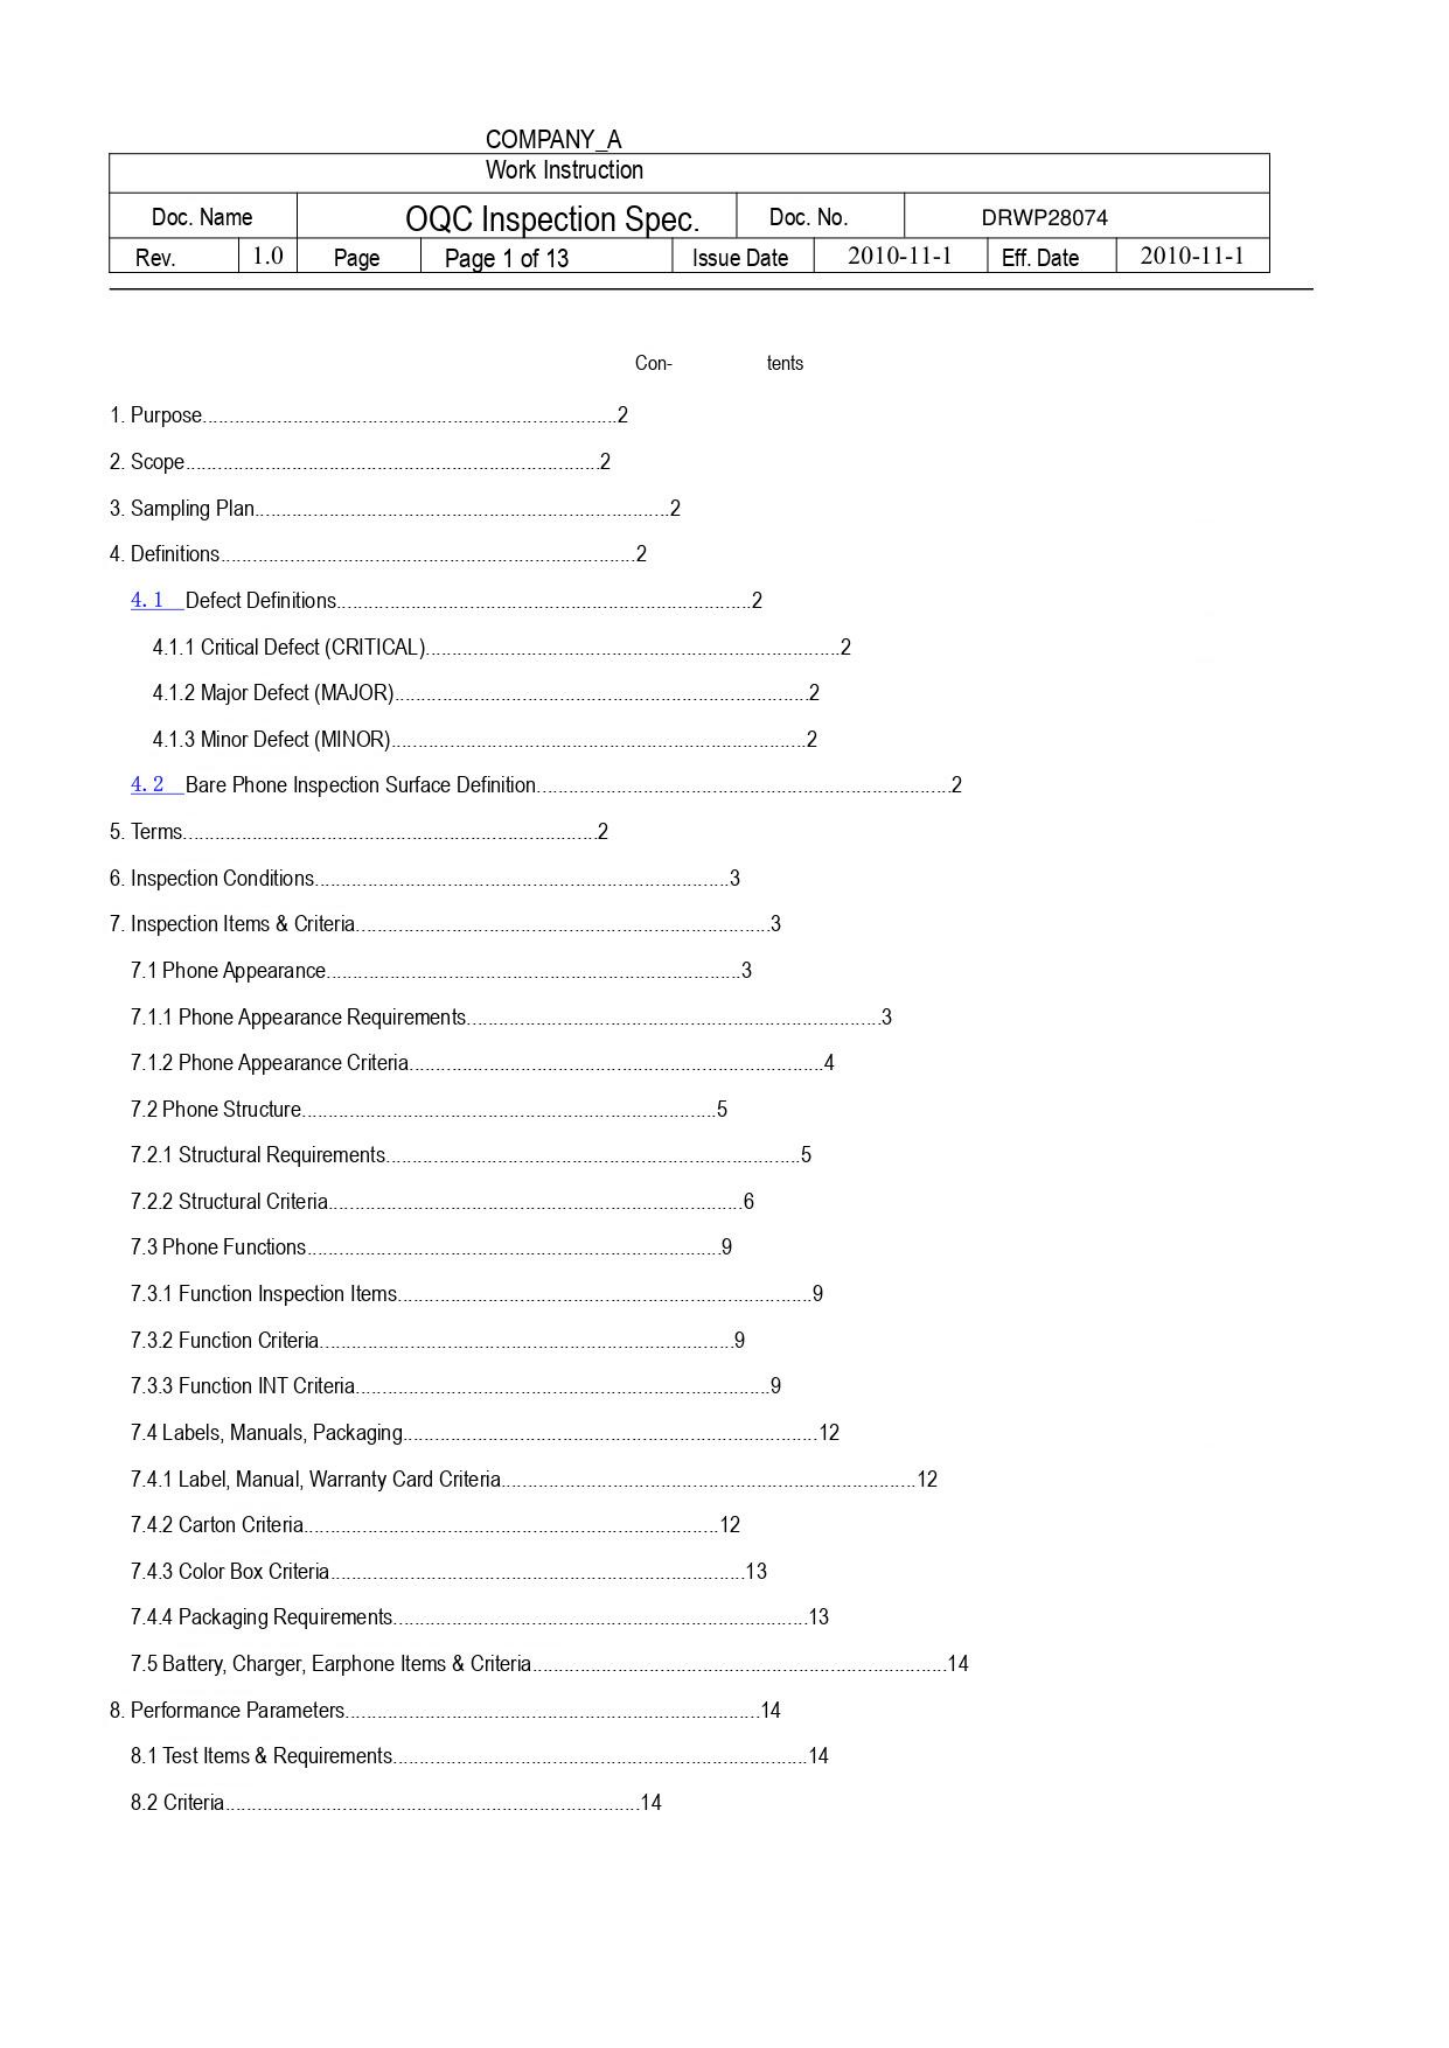COMPANY_A

| Work Instruction | | | | | | | |
|---|---|---|---|---|---|---|---|
| Doc. Name | | OQC Inspection Spec. | | Doc. No. | | DRWP28074 | |
| Rev. | 1.0 | Page | Page 1 of 13 | Issue Date | 2010-11-1 | Eff. Date | 2010-11-1 |

Con- tents

1. Purpose.....2

2. Scope.....2

3. Sampling Plan.....2

4. Definitions.....2

4. 1 Defect Definitions.....2

4.1.1 Critical Defect (CRITICAL).....2

4.1.2 Major Defect (MAJOR).....2

4.1.3 Minor Defect (MINOR).....2

4. 2 Bare Phone Inspection Surface Definition.....2

5. Terms.....2

6. Inspection Conditions.....3

7. Inspection Items & Criteria.....3

7.1 Phone Appearance.....3

7.1.1 Phone Appearance Requirements.....3

7.1.2 Phone Appearance Criteria.....4

7.2 Phone Structure.....5

7.2.1 Structural Requirements.....5

7.2.2 Structural Criteria.....6

7.3 Phone Functions.....9

7.3.1 Function Inspection Items.....9

7.3.2 Function Criteria.....9

7.3.3 Function INT Criteria.....9

7.4 Labels, Manuals, Packaging.....12

7.4.1 Label, Manual, Warranty Card Criteria.....12

7.4.2 Carton Criteria.....12

7.4.3 Color Box Criteria.....13

7.4.4 Packaging Requirements.....13

7.5 Battery, Charger, Earphone Items & Criteria.....14

8. Performance Parameters.....14

8.1 Test Items & Requirements.....14

8.2 Criteria.....14
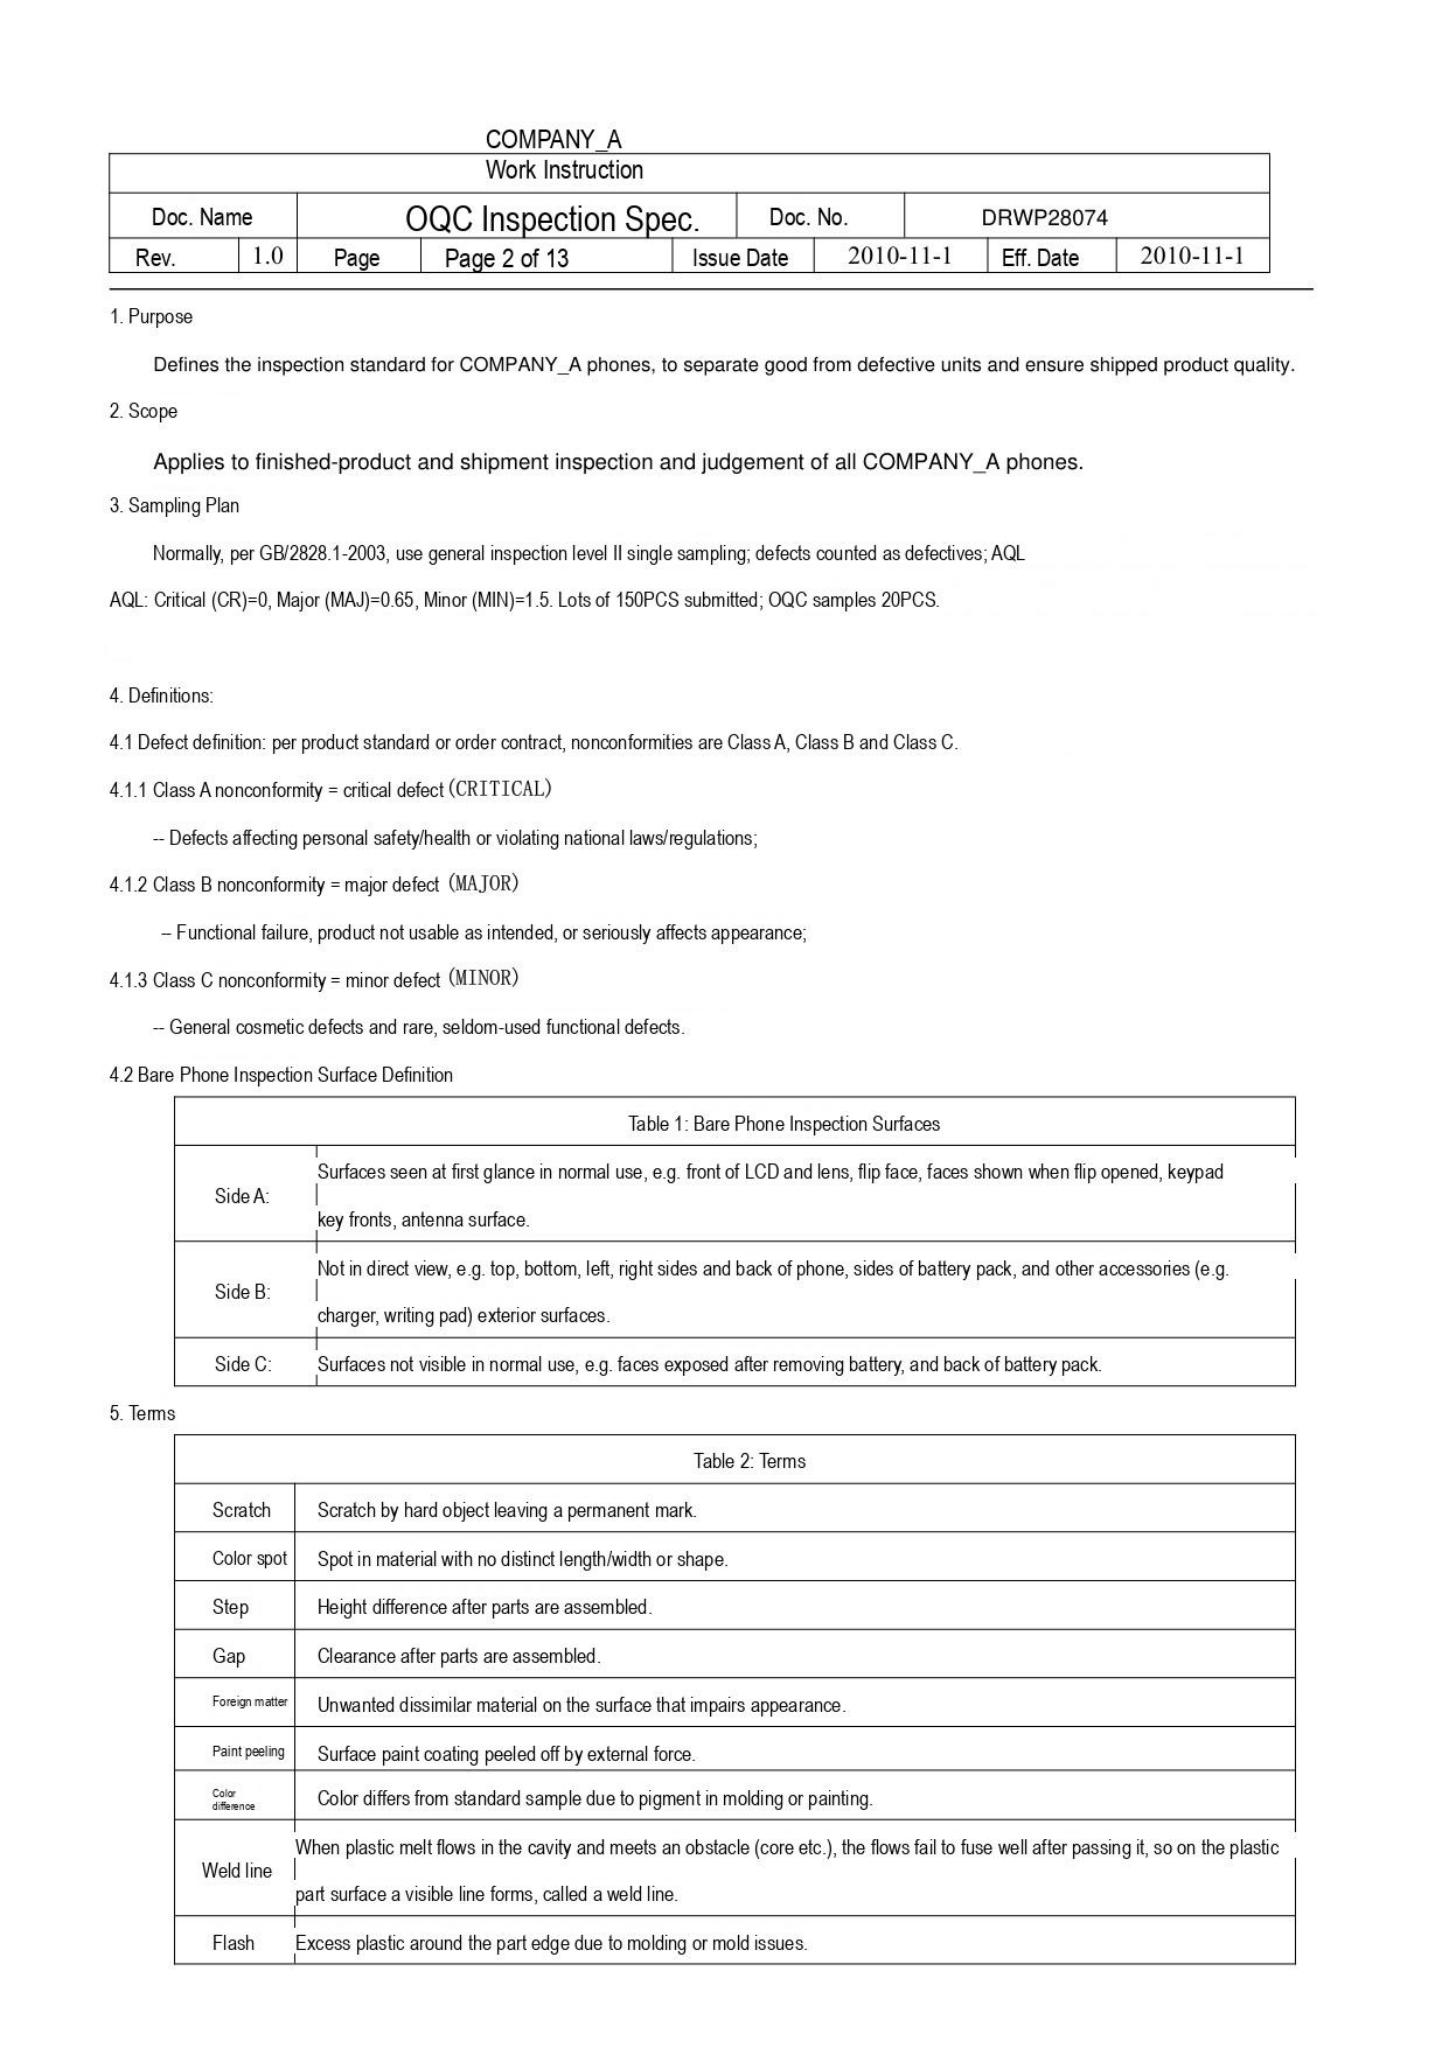COMPANY_A

| Work Instruction | | | | | | | |
|---|---|---|---|---|---|---|---|
| Doc. Name | | OQC Inspection Spec. | | Doc. No. | DRWP28074 | | |
| Rev. | 1.0 | Page | Page 2 of 13 | Issue Date | 2010-11-1 | Eff. Date | 2010-11-1 |

1. Purpose

Defines the inspection standard for COMPANY_A phones, to separate good from defective units and ensure shipped product quality.

2. Scope

Applies to finished-product and shipment inspection and judgement of all COMPANY_A phones.

3. Sampling Plan

Normally, per GB/2828.1-2003, use general inspection level II single sampling; defects counted as defectives; AQL

AQL: Critical (CR)=0, Major (MAJ)=0.65, Minor (MIN)=1.5. Lots of 150PCS submitted; OQC samples 20PCS.

4. Definitions:

4.1 Defect definition: per product standard or order contract, nonconformities are Class A, Class B and Class C.

4.1.1 Class A nonconformity = critical defect (CRITICAL)

-- Defects affecting personal safety/health or violating national laws/regulations;

4.1.2 Class B nonconformity = major defect (MAJOR)

– Functional failure, product not usable as intended, or seriously affects appearance;

4.1.3 Class C nonconformity = minor defect (MINOR)

-- General cosmetic defects and rare, seldom-used functional defects.

4.2 Bare Phone Inspection Surface Definition

| Table 1: Bare Phone Inspection Surfaces | |
|---|---|
| Side A: | Surfaces seen at first glance in normal use, e.g. front of LCD and lens, flip face, faces shown when flip opened, keypad key fronts, antenna surface. |
| Side B: | Not in direct view, e.g. top, bottom, left, right sides and back of phone, sides of battery pack, and other accessories (e.g. charger, writing pad) exterior surfaces. |
| Side C: | Surfaces not visible in normal use, e.g. faces exposed after removing battery, and back of battery pack. |

5. Terms

| Table 2: Terms | |
|---|---|
| Scratch | Scratch by hard object leaving a permanent mark. |
| Color spot | Spot in material with no distinct length/width or shape. |
| Step | Height difference after parts are assembled. |
| Gap | Clearance after parts are assembled. |
| Foreign matter | Unwanted dissimilar material on the surface that impairs appearance. |
| Paint peeling | Surface paint coating peeled off by external force. |
| Color difference | Color differs from standard sample due to pigment in molding or painting. |
| Weld line | When plastic melt flows in the cavity and meets an obstacle (core etc.), the flows fail to fuse well after passing it, so on the plastic part surface a visible line forms, called a weld line. |
| Flash | Excess plastic around the part edge due to molding or mold issues. |
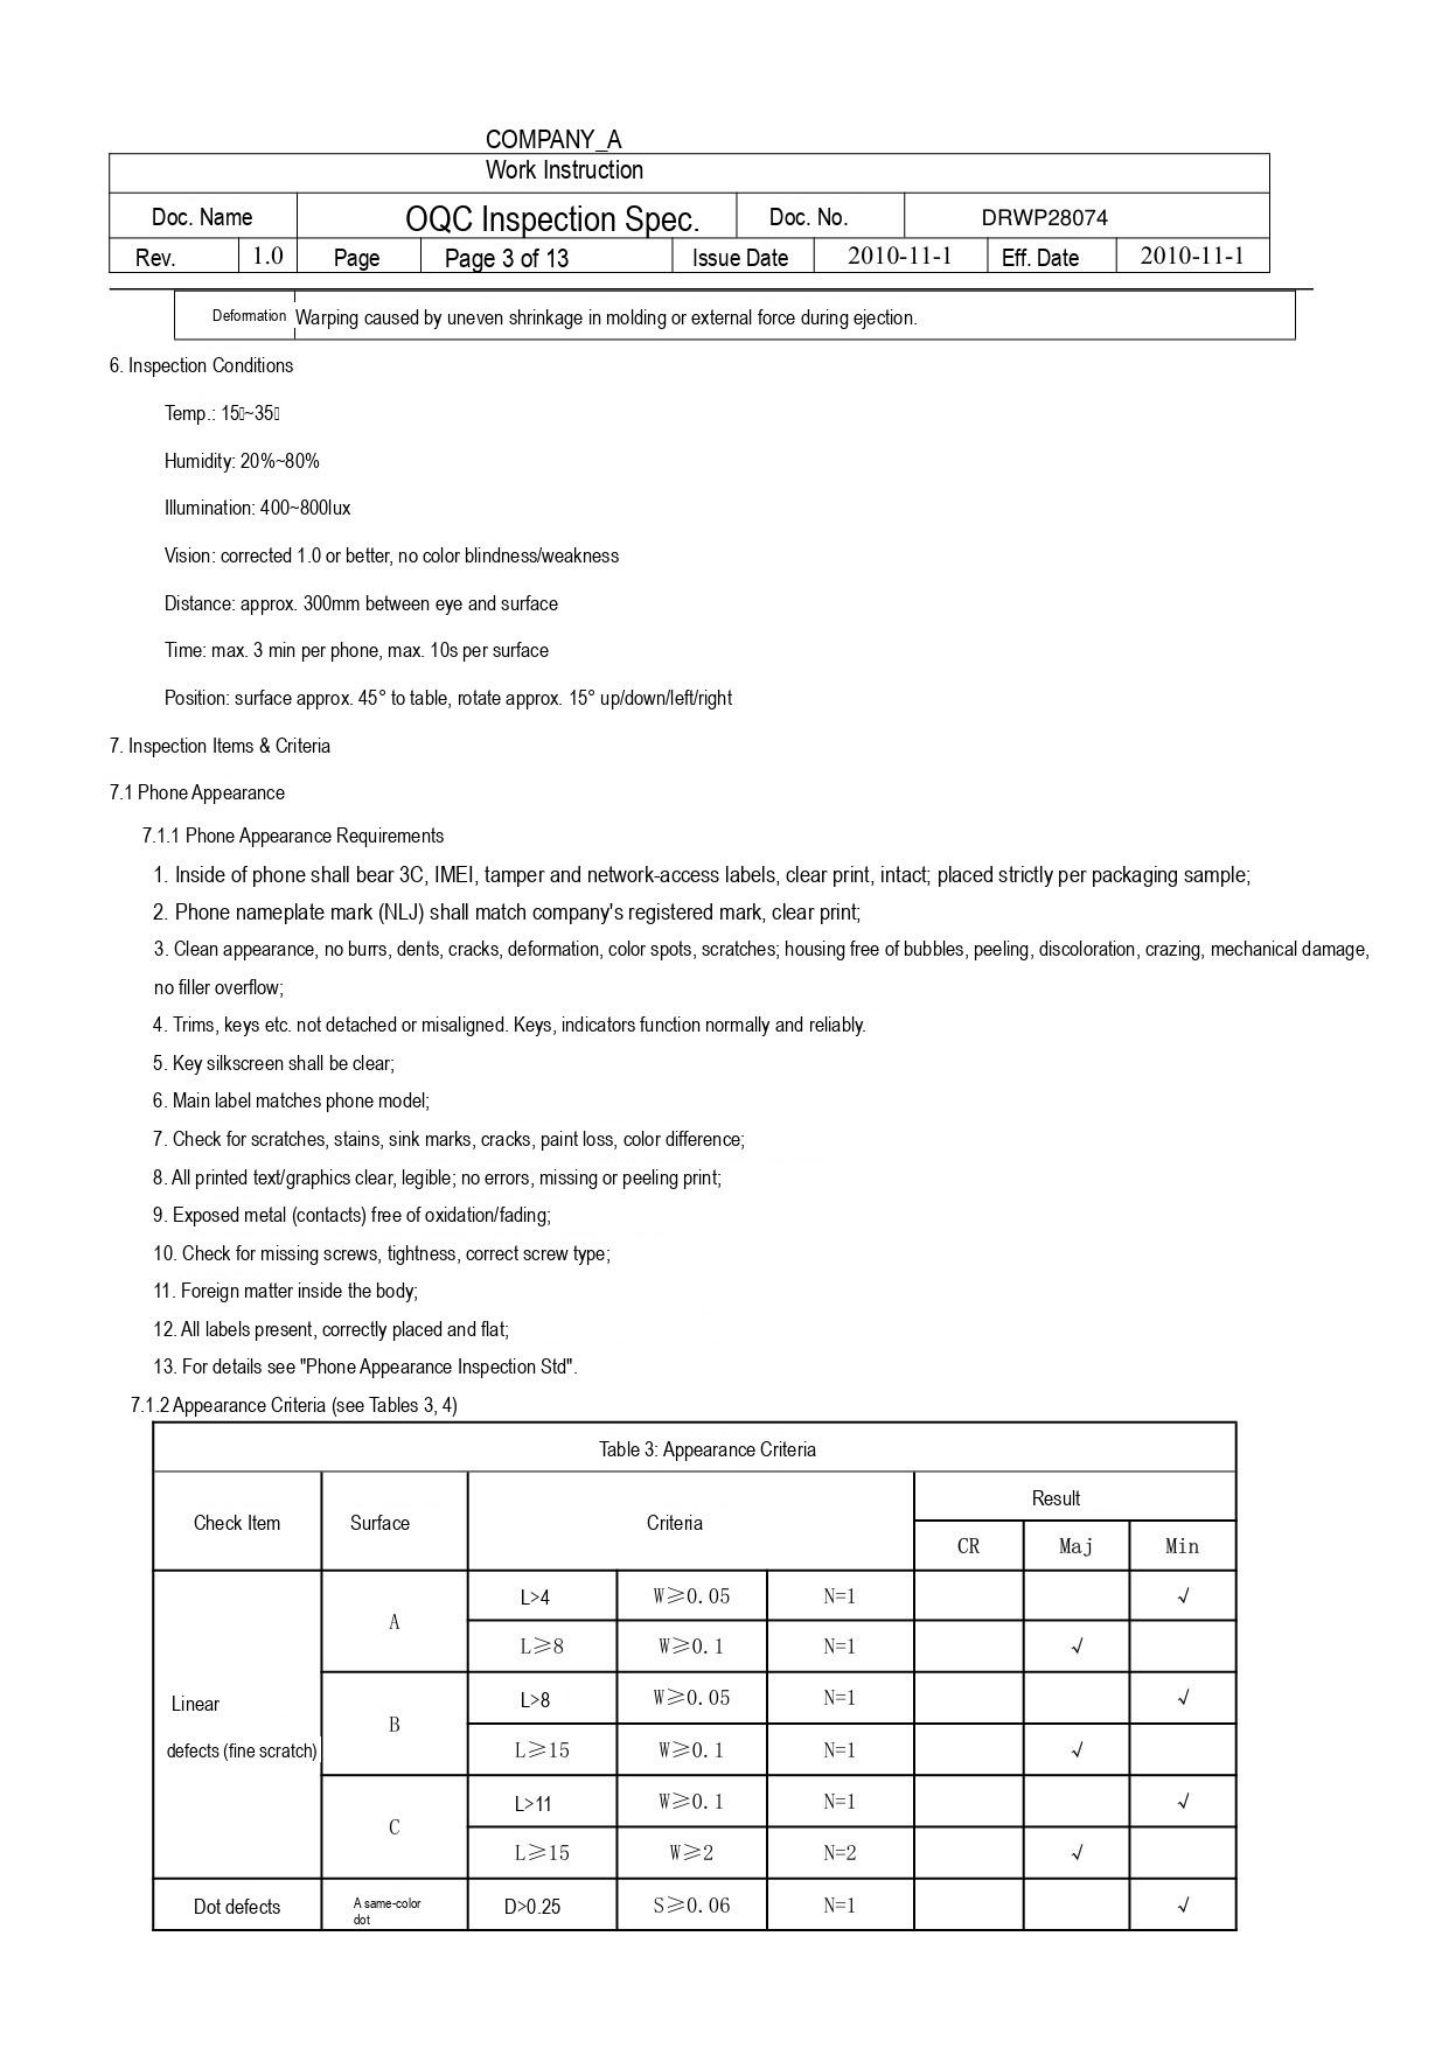COMPANY_A

| Work Instruction | | | | | | | |
|---|---|---|---|---|---|---|---|
| Doc. Name | | OQC Inspection Spec. | | Doc. No. | DRWP28074 | | |
| Rev. | 1.0 | Page | Page 3 of 13 | Issue Date | 2010-11-1 | Eff. Date | 2010-11-1 |

| Deformation | Warping caused by uneven shrinkage in molding or external force during ejection. |
|---|---|

6. Inspection Conditions

Temp.: 15~35

Humidity: 20%~80%

Illumination: 400~800lux

Vision: corrected 1.0 or better, no color blindness/weakness

Distance: approx. 300mm between eye and surface

Time: max. 3 min per phone, max. 10s per surface

Position: surface approx. 45° to table, rotate approx. 15° up/down/left/right

7. Inspection Items & Criteria

7.1 Phone Appearance

7.1.1 Phone Appearance Requirements

1. Inside of phone shall bear 3C, IMEI, tamper and network-access labels, clear print, intact; placed strictly per packaging sample;

2. Phone nameplate mark (NLJ) shall match company's registered mark, clear print;

3. Clean appearance, no burrs, dents, cracks, deformation, color spots, scratches; housing free of bubbles, peeling, discoloration, crazing, mechanical damage, no filler overflow;

4. Trims, keys etc. not detached or misaligned. Keys, indicators function normally and reliably.

5. Key silkscreen shall be clear;

6. Main label matches phone model;

7. Check for scratches, stains, sink marks, cracks, paint loss, color difference;

8. All printed text/graphics clear, legible; no errors, missing or peeling print;

9. Exposed metal (contacts) free of oxidation/fading;

10. Check for missing screws, tightness, correct screw type;

11. Foreign matter inside the body;

12. All labels present, correctly placed and flat;

13. For details see "Phone Appearance Inspection Std".

7.1.2 Appearance Criteria (see Tables 3, 4)

Table 3: Appearance Criteria

| Check Item | Surface | Criteria | | | Result CR | Result Maj | Result Min |
|---|---|---|---|---|---|---|---|
| Linear defects (fine scratch) | A | L>4 | W≥0.05 | N=1 | | | √ |
| | | L≥8 | W≥0.1 | N=1 | | √ | |
| | B | L>8 | W≥0.05 | N=1 | | | √ |
| | | L≥15 | W≥0.1 | N=1 | | √ | |
| | C | L>11 | W≥0.1 | N=1 | | | √ |
| | | L≥15 | W≥2 | N=2 | | √ | |
| Dot defects | A same-color dot | D>0.25 | S≥0.06 | N=1 | | | √ |
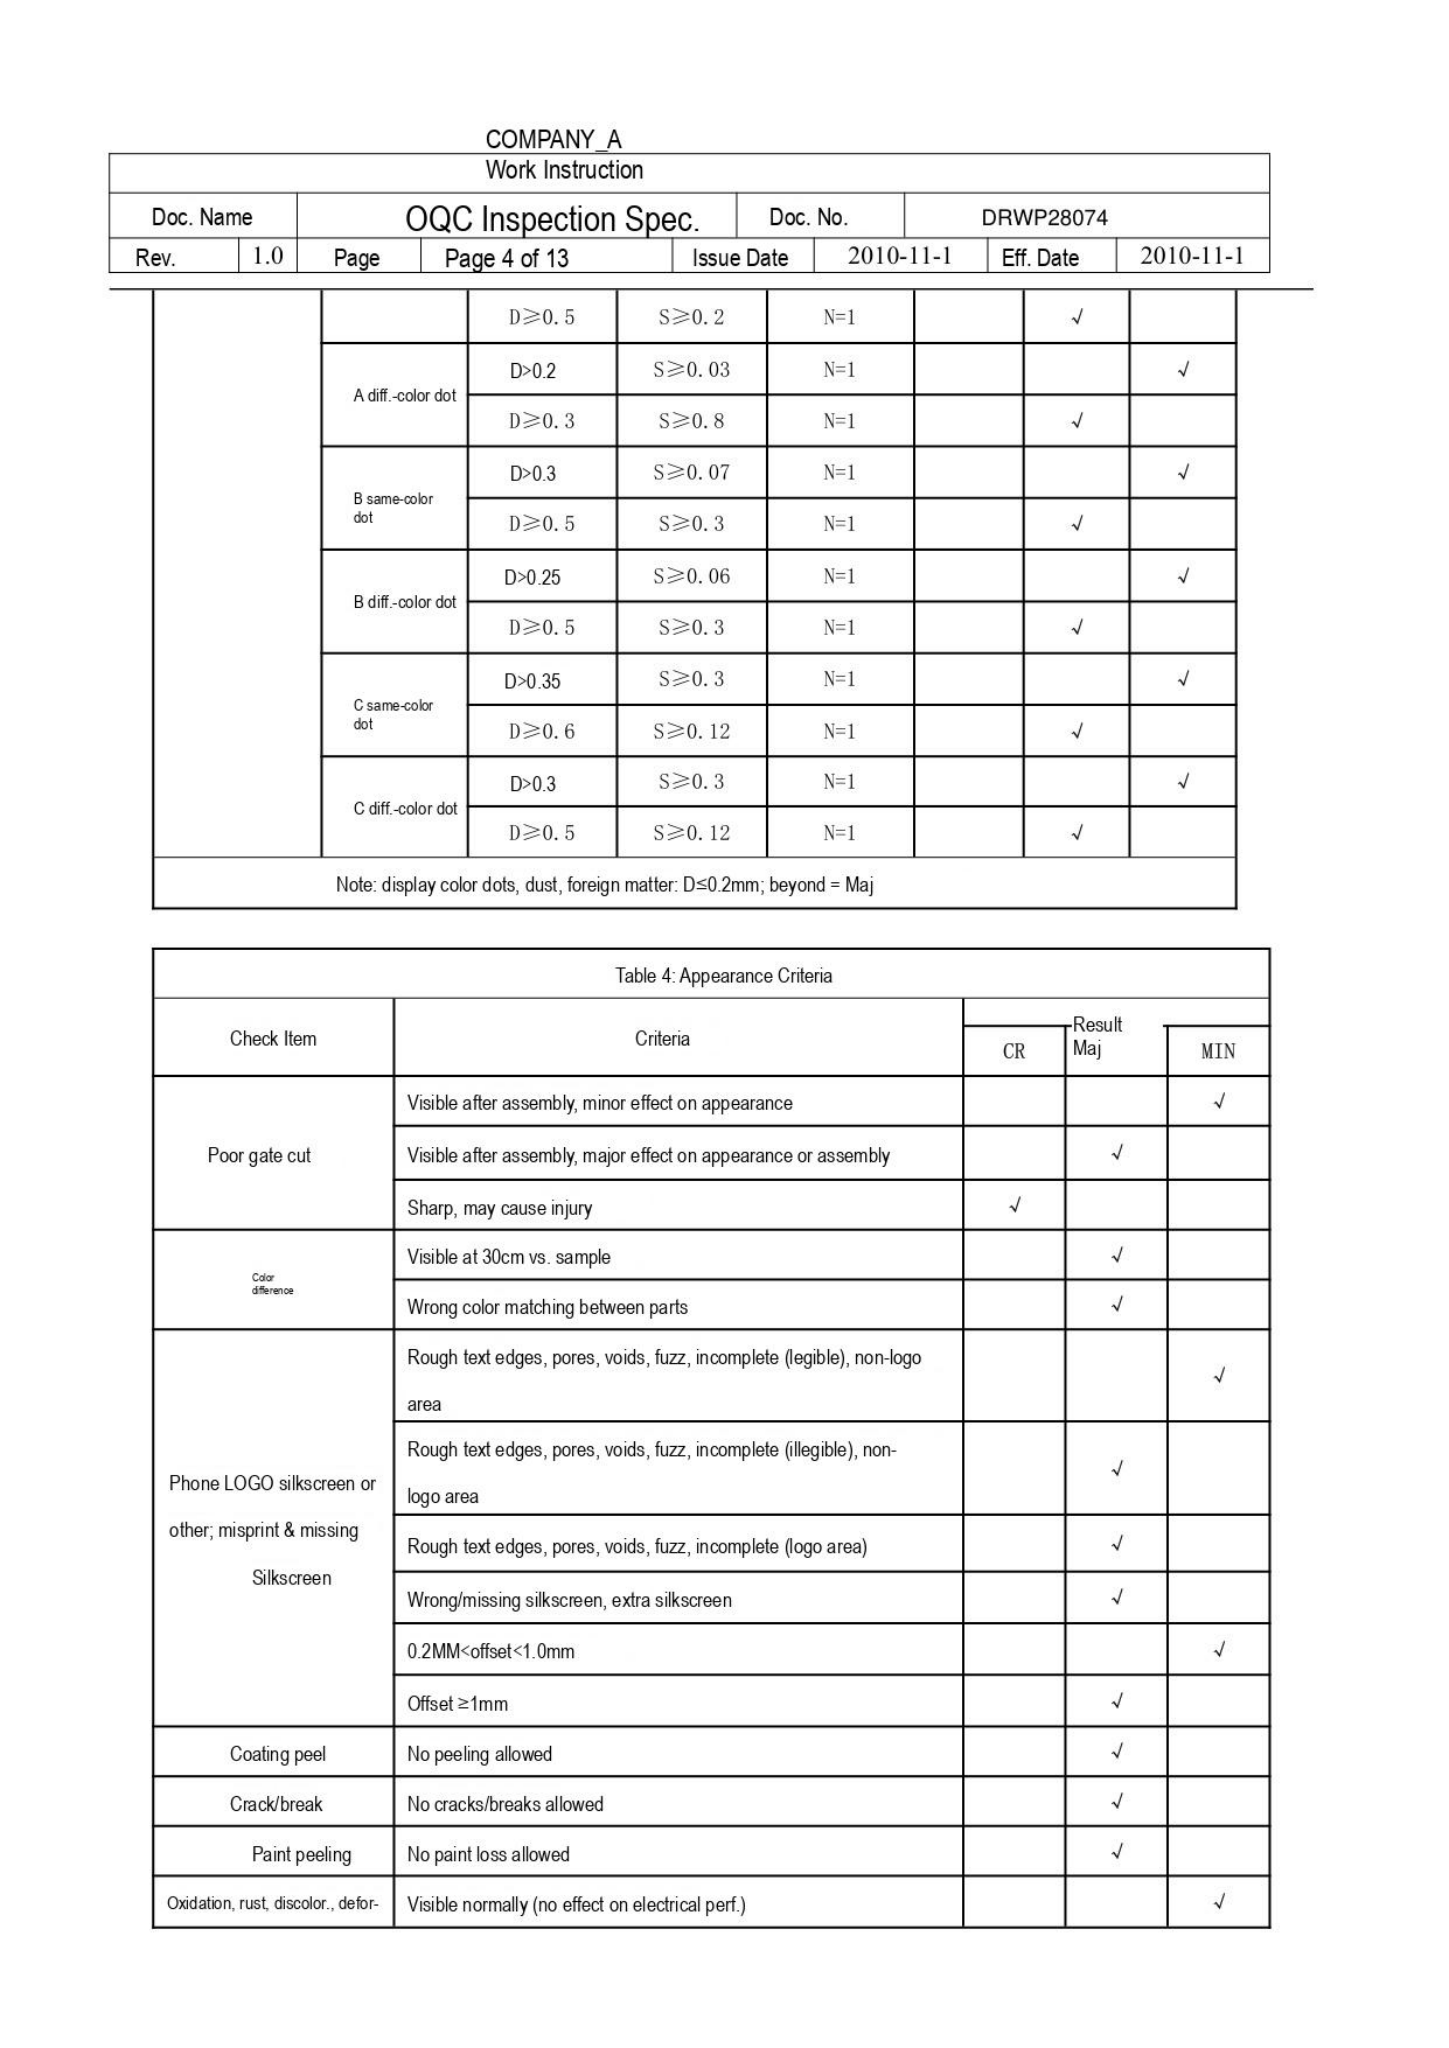COMPANY_A

| Work Instruction | | | | | | | |
|---|---|---|---|---|---|---|---|
| Doc. Name | | OQC Inspection Spec. | | Doc. No. | | DRWP28074 | |
| Rev. | 1.0 | Page | Page 4 of 13 | Issue Date | 2010-11-1 | Eff. Date | 2010-11-1 |

| | | | | | | | |
|---|---|---|---|---|---|---|---|
| | | D≥0.5 | S≥0.2 | N=1 | | √ | |
| | A diff.-color dot | D>0.2 | S≥0.03 | N=1 | | | √ |
| | | D≥0.3 | S≥0.8 | N=1 | | √ | |
| | B same-color dot | D>0.3 | S≥0.07 | N=1 | | | √ |
| | | D≥0.5 | S≥0.3 | N=1 | | √ | |
| | B diff.-color dot | D>0.25 | S≥0.06 | N=1 | | | √ |
| | | D≥0.5 | S≥0.3 | N=1 | | √ | |
| | C same-color dot | D>0.35 | S≥0.3 | N=1 | | | √ |
| | | D≥0.6 | S≥0.12 | N=1 | | √ | |
| | C diff.-color dot | D>0.3 | S≥0.3 | N=1 | | | √ |
| | | D≥0.5 | S≥0.12 | N=1 | | √ | |
| Note: display color dots, dust, foreign matter: D≤0.2mm; beyond = Maj | | | | | | | |

Table 4: Appearance Criteria

| Check Item | Criteria | Result CR | Result Maj | Result MIN |
|---|---|---|---|---|
| Poor gate cut | Visible after assembly, minor effect on appearance | | | √ |
| | Visible after assembly, major effect on appearance or assembly | | √ | |
| | Sharp, may cause injury | √ | | |
| Color difference | Visible at 30cm vs. sample | | √ | |
| | Wrong color matching between parts | | √ | |
| Phone LOGO silkscreen or other; misprint & missing Silkscreen | Rough text edges, pores, voids, fuzz, incomplete (legible), non-logo area | | | √ |
| | Rough text edges, pores, voids, fuzz, incomplete (illegible), non-logo area | | √ | |
| | Rough text edges, pores, voids, fuzz, incomplete (logo area) | | √ | |
| | Wrong/missing silkscreen, extra silkscreen | | √ | |
| | 0.2MM<offset<1.0mm | | | √ |
| | Offset ≥1mm | | √ | |
| Coating peel | No peeling allowed | | √ | |
| Crack/break | No cracks/breaks allowed | | √ | |
| Paint peeling | No paint loss allowed | | √ | |
| Oxidation, rust, discolor., defor- | Visible normally (no effect on electrical perf.) | | | √ |
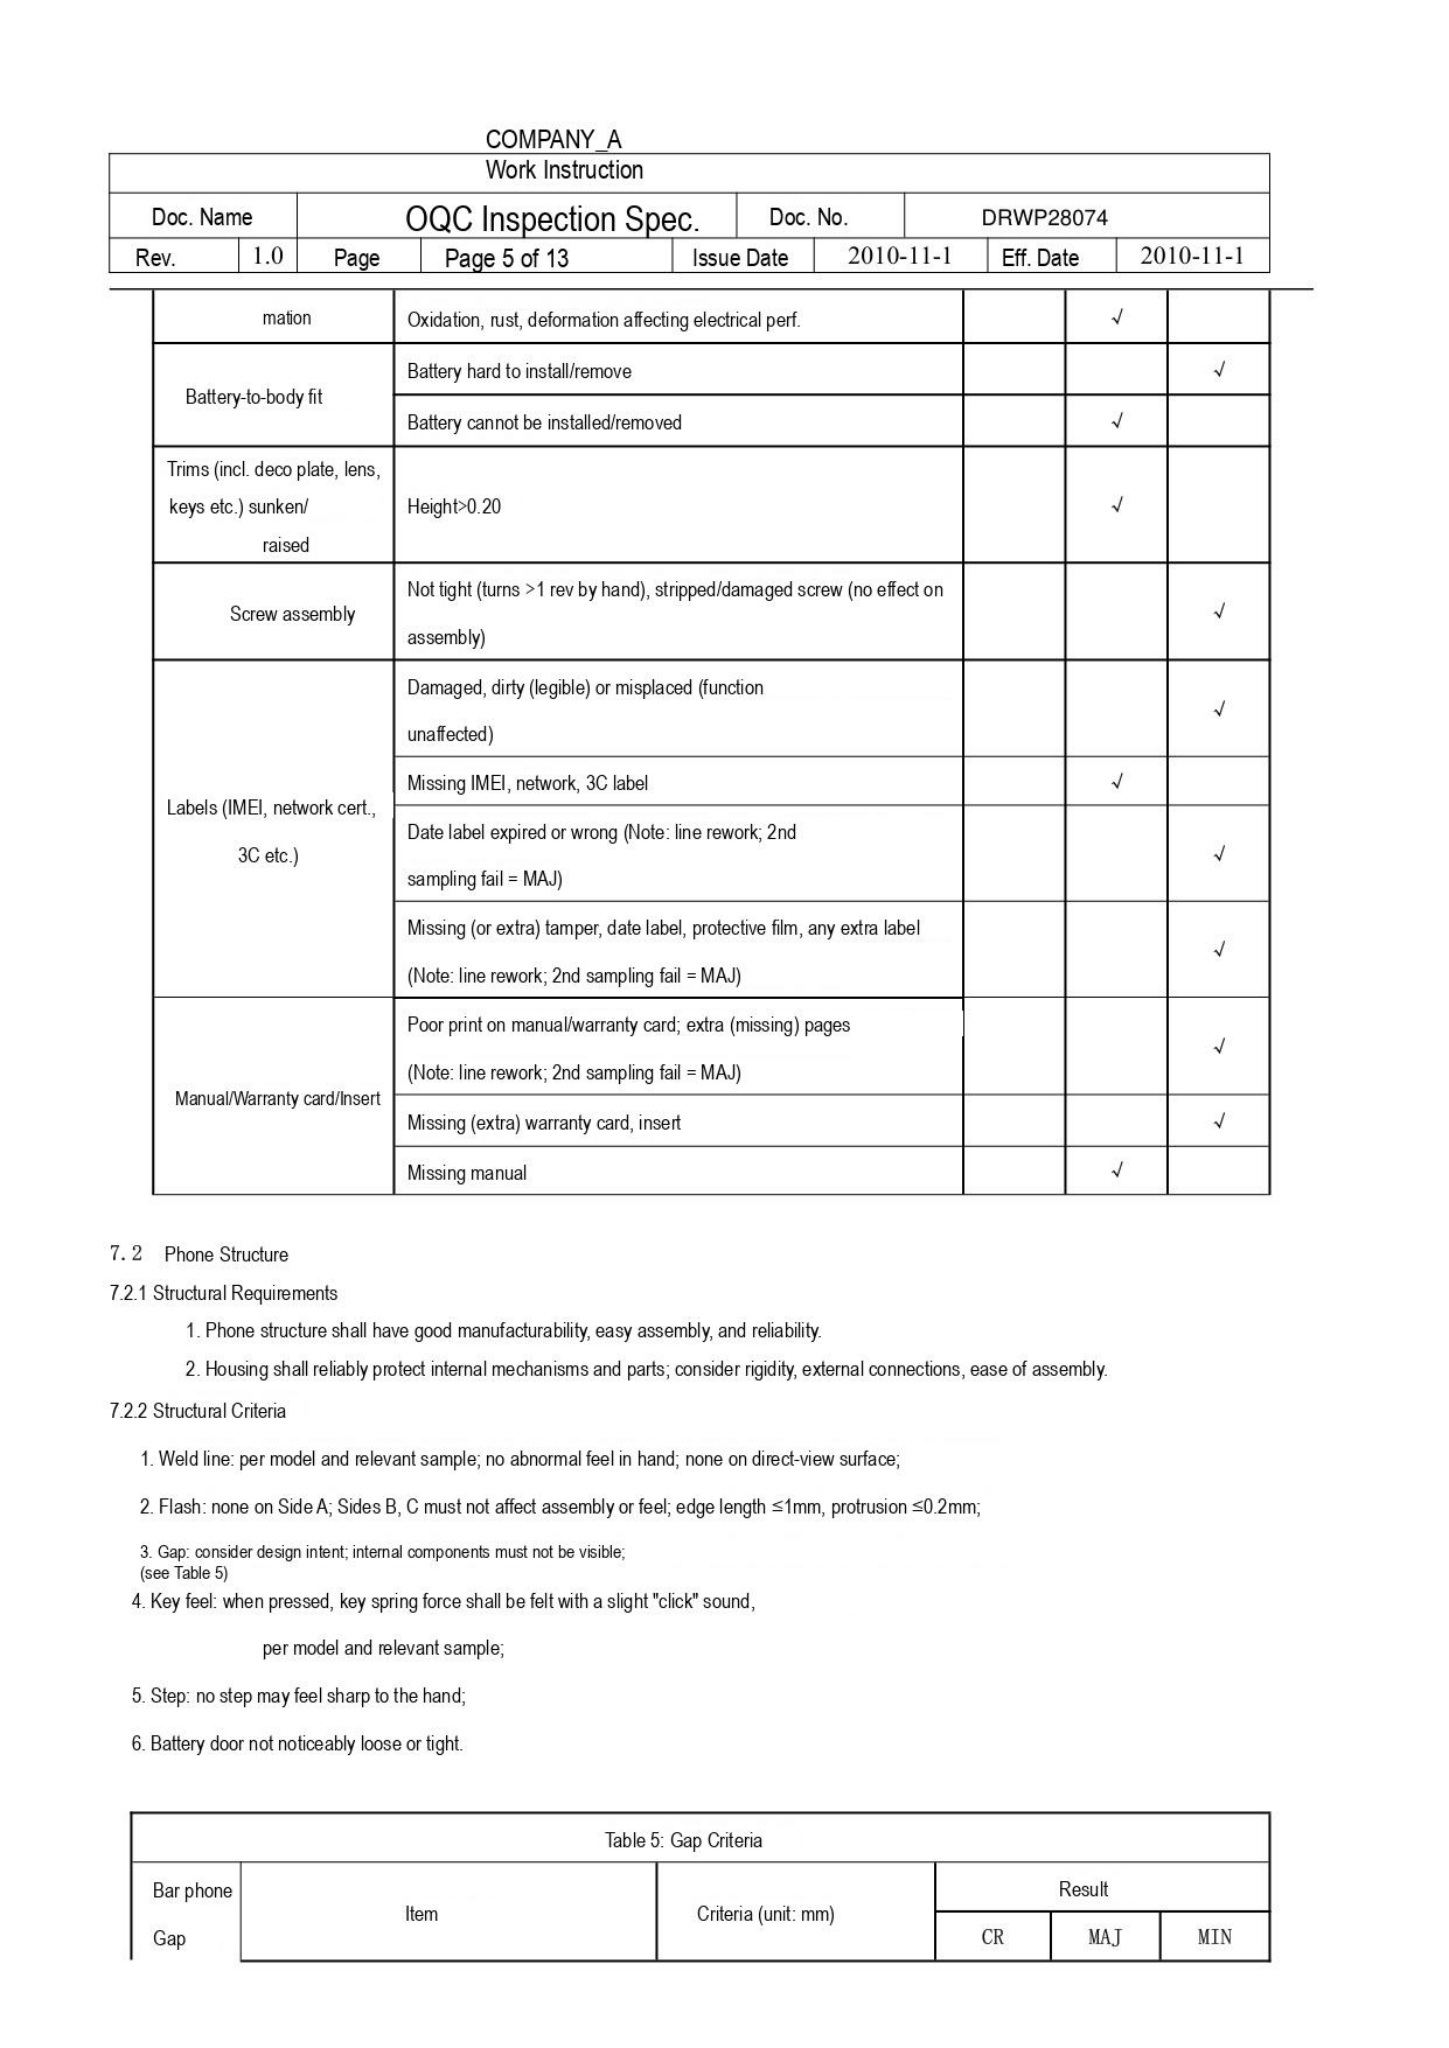COMPANY_A

| Work Instruction | | | | | | | |
|---|---|---|---|---|---|---|---|
| Doc. Name | | OQC Inspection Spec. | | Doc. No. | | DRWP28074 | |
| Rev. | 1.0 | Page | Page 5 of 13 | Issue Date | 2010-11-1 | Eff. Date | 2010-11-1 |

| | | | | |
|---|---|---|---|---|
| mation | Oxidation, rust, deformation affecting electrical perf. | | √ | |
| Battery-to-body fit | Battery hard to install/remove | | | √ |
| | Battery cannot be installed/removed | | √ | |
| Trims (incl. deco plate, lens, keys etc.) sunken/ raised | Height>0.20 | | √ | |
| Screw assembly | Not tight (turns >1 rev by hand), stripped/damaged screw (no effect on assembly) | | | √ |
| Labels (IMEI, network cert., 3C etc.) | Damaged, dirty (legible) or misplaced (function unaffected) | | | √ |
| | Missing IMEI, network, 3C label | | √ | |
| | Date label expired or wrong (Note: line rework; 2nd sampling fail = MAJ) | | | √ |
| | Missing (or extra) tamper, date label, protective film, any extra label (Note: line rework; 2nd sampling fail = MAJ) | | | √ |
| Manual/Warranty card/Insert | Poor print on manual/warranty card; extra (missing) pages (Note: line rework; 2nd sampling fail = MAJ) | | | √ |
| | Missing (extra) warranty card, insert | | | √ |
| | Missing manual | | √ | |

7.2 Phone Structure

7.2.1 Structural Requirements

1. Phone structure shall have good manufacturability, easy assembly, and reliability.

2. Housing shall reliably protect internal mechanisms and parts; consider rigidity, external connections, ease of assembly.

7.2.2 Structural Criteria

1. Weld line: per model and relevant sample; no abnormal feel in hand; none on direct-view surface;

2. Flash: none on Side A; Sides B, C must not affect assembly or feel; edge length ≤1mm, protrusion ≤0.2mm;

3. Gap: consider design intent; internal components must not be visible;
(see Table 5)

4. Key feel: when pressed, key spring force shall be felt with a slight "click" sound,

per model and relevant sample;

5. Step: no step may feel sharp to the hand;

6. Battery door not noticeably loose or tight.

| Table 5: Gap Criteria | | | | | |
|---|---|---|---|---|---|
| Bar phone Gap | Item | Criteria (unit: mm) | Result | | |
| | | | CR | MAJ | MIN |
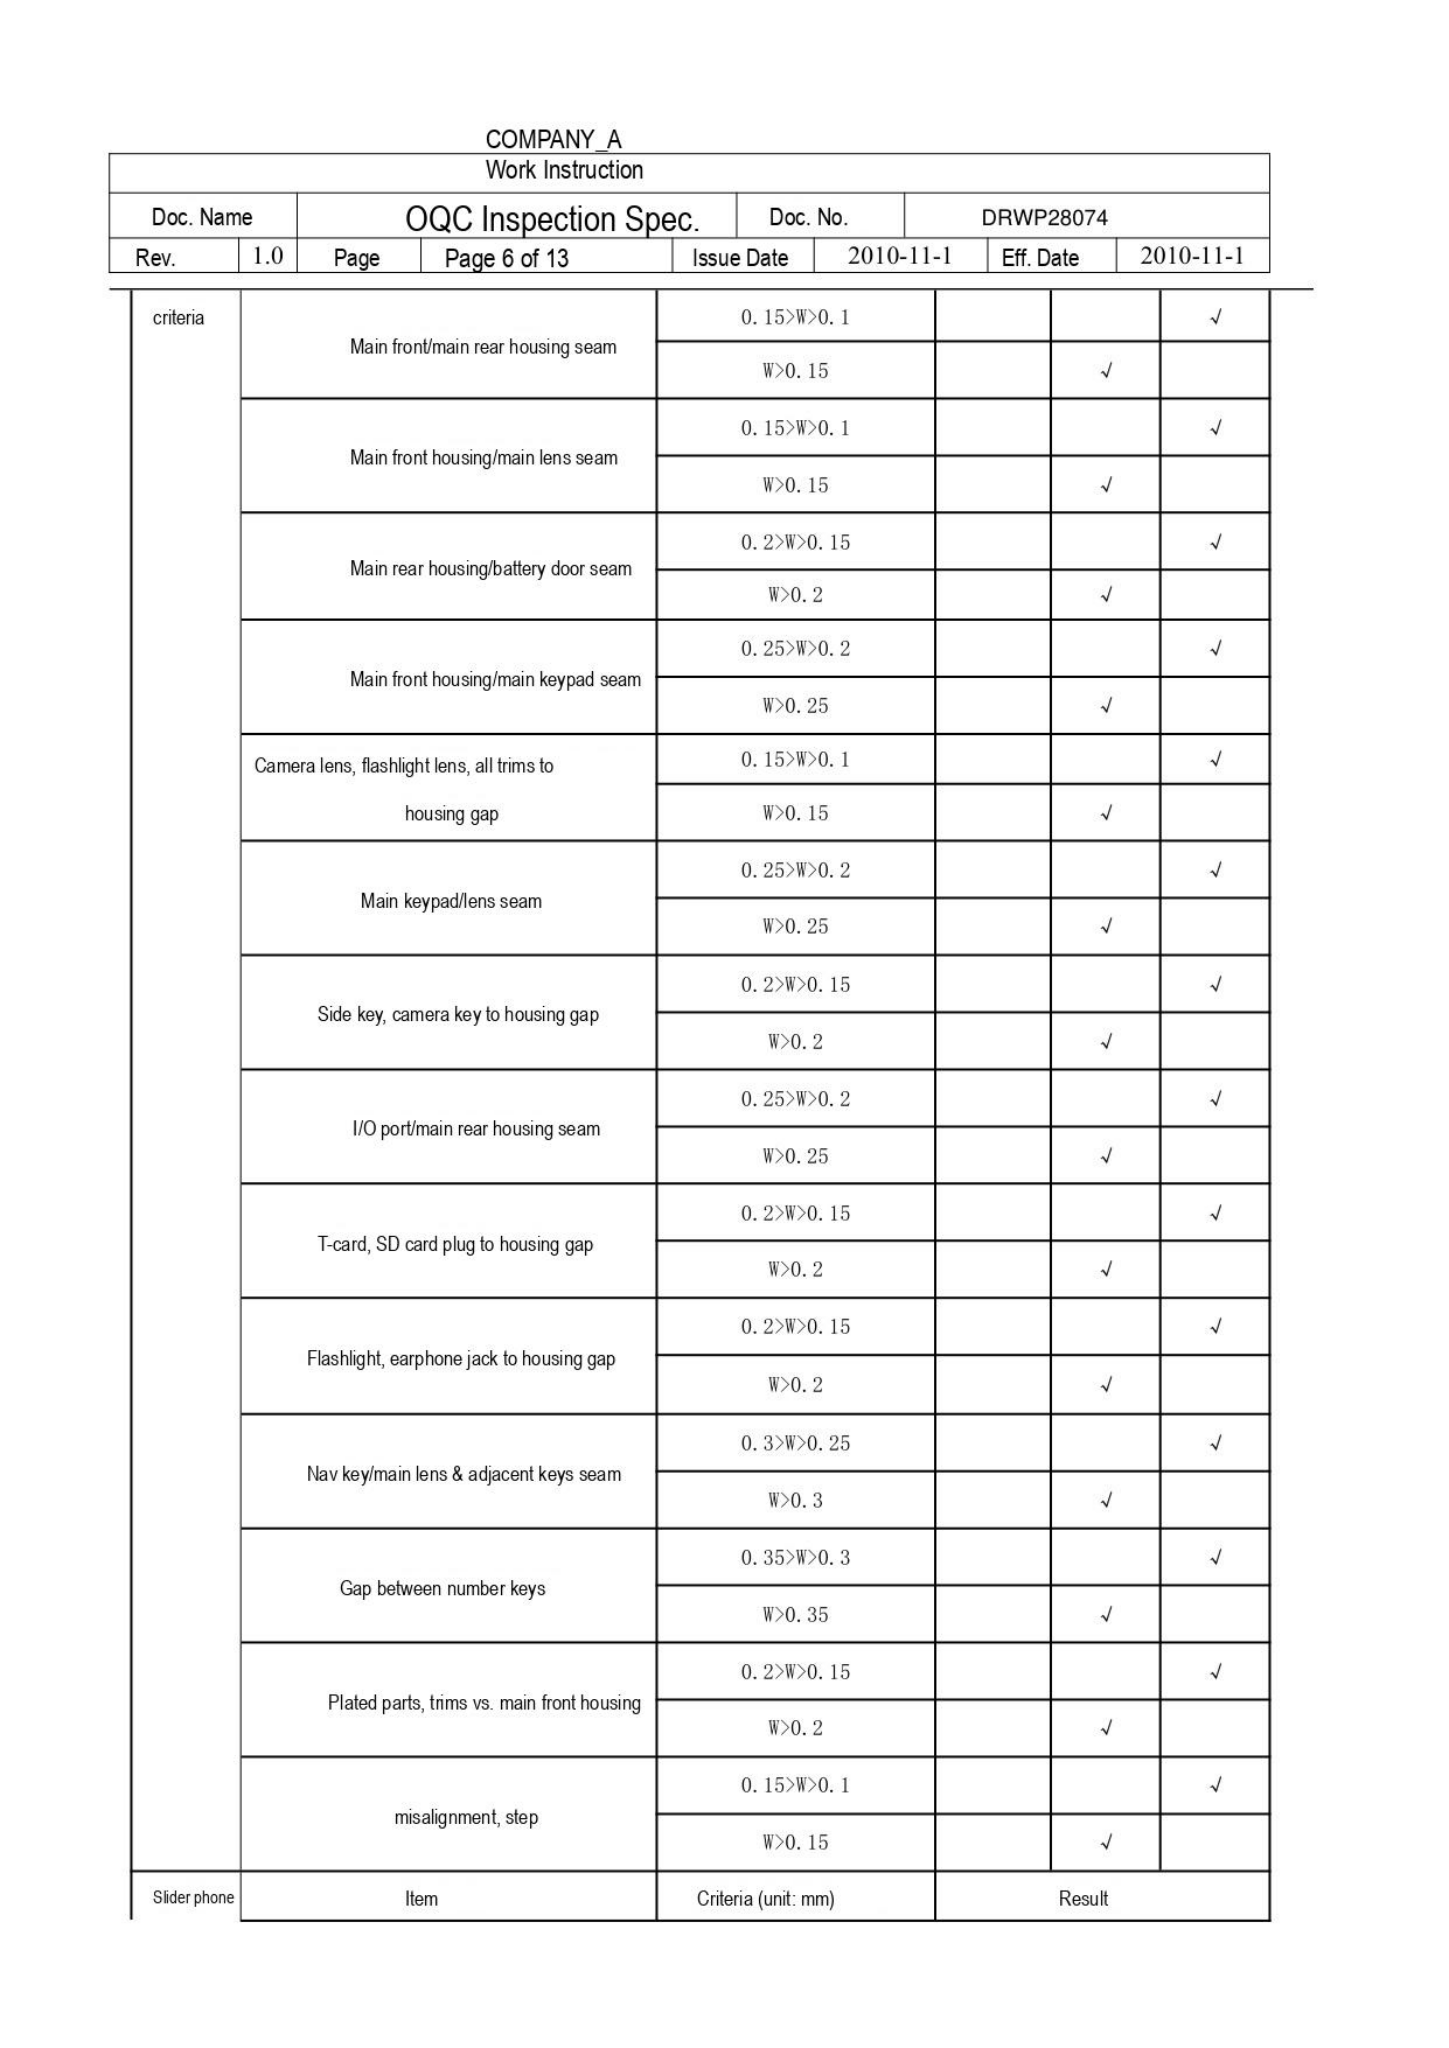COMPANY_A

| Work Instruction | | | | | | | |
|---|---|---|---|---|---|---|---|
| Doc. Name | | OQC Inspection Spec. | | Doc. No. | | DRWP28074 | |
| Rev. | 1.0 | Page | Page 6 of 13 | Issue Date | 2010-11-1 | Eff. Date | 2010-11-1 |

| | | | | | |
|---|---|---|---|---|---|
| criteria | Main front/main rear housing seam | 0. 15>W>0. 1 | | | √ |
| | | W>0. 15 | | √ | |
| | Main front housing/main lens seam | 0. 15>W>0. 1 | | | √ |
| | | W>0. 15 | | √ | |
| | Main rear housing/battery door seam | 0. 2>W>0. 15 | | | √ |
| | | W>0. 2 | | √ | |
| | Main front housing/main keypad seam | 0. 25>W>0. 2 | | | √ |
| | | W>0. 25 | | √ | |
| | Camera lens, flashlight lens, all trims to housing gap | 0. 15>W>0. 1 | | | √ |
| | | W>0. 15 | | √ | |
| | Main keypad/lens seam | 0. 25>W>0. 2 | | | √ |
| | | W>0. 25 | | √ | |
| | Side key, camera key to housing gap | 0. 2>W>0. 15 | | | √ |
| | | W>0. 2 | | √ | |
| | I/O port/main rear housing seam | 0. 25>W>0. 2 | | | √ |
| | | W>0. 25 | | √ | |
| | T-card, SD card plug to housing gap | 0. 2>W>0. 15 | | | √ |
| | | W>0. 2 | | √ | |
| | Flashlight, earphone jack to housing gap | 0. 2>W>0. 15 | | | √ |
| | | W>0. 2 | | √ | |
| | Nav key/main lens & adjacent keys seam | 0. 3>W>0. 25 | | | √ |
| | | W>0. 3 | | √ | |
| | Gap between number keys | 0. 35>W>0. 3 | | | √ |
| | | W>0. 35 | | √ | |
| | Plated parts, trims vs. main front housing | 0. 2>W>0. 15 | | | √ |
| | | W>0. 2 | | √ | |
| | misalignment, step | 0. 15>W>0. 1 | | | √ |
| | | W>0. 15 | | √ | |
| Slider phone | Item | Criteria (unit: mm) | Result | | |